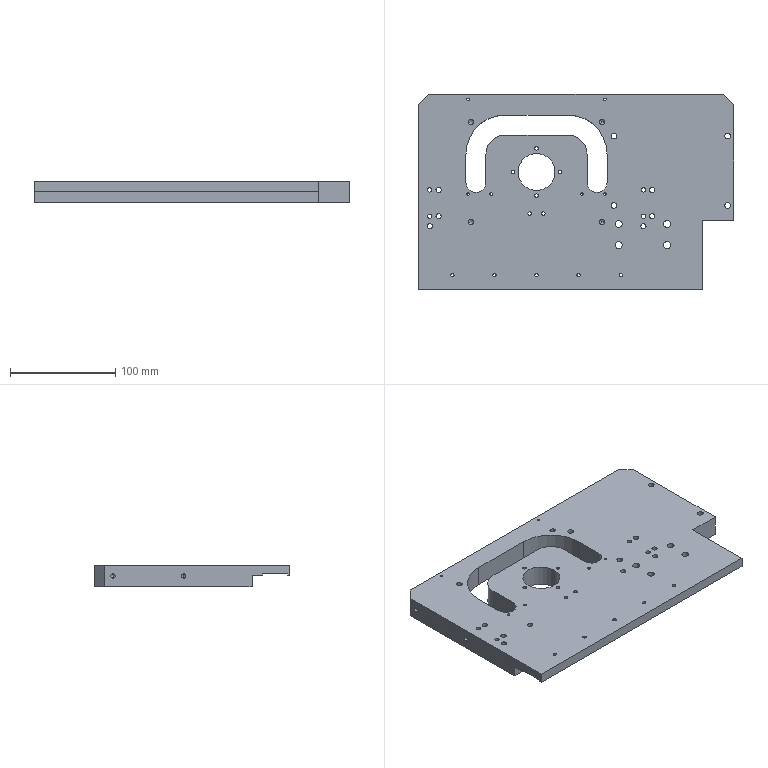Part | STEP file | 11-FG-E00111 | 1 solid | 164 faces | box 300 x 186 x 20 mm | volume 846486 mm3 | cylinder 114 | plane 30 | cone 20 | commonest cylinder face diameters 3.3 x22 5 x20 2.5 x16 4.2 x16 5.5 x8 6.6 x8